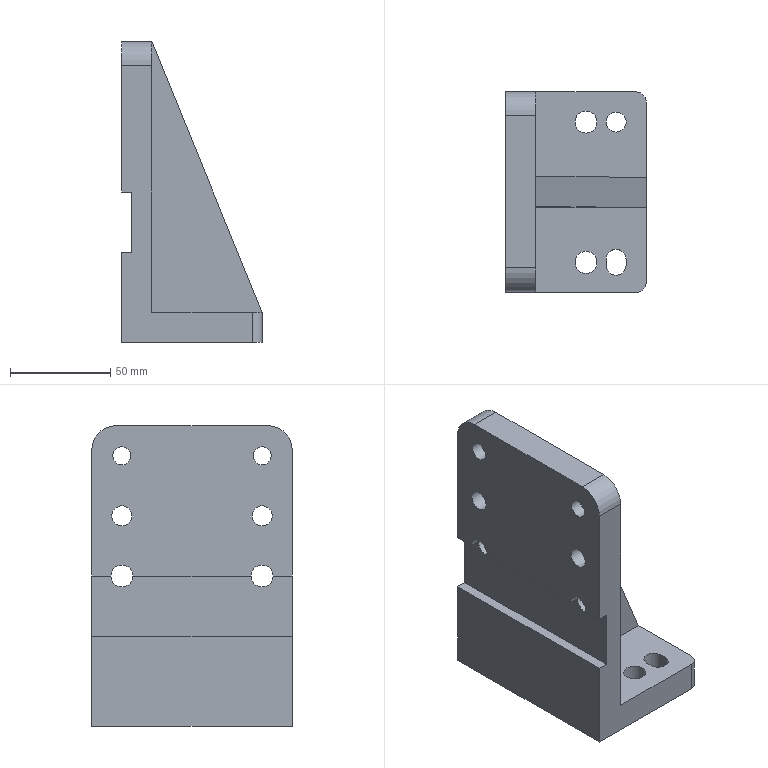Part | NX | features 5003_014_C-AIKK150-70 2 | 1 solid | 40 faces | box 70 x 100 x 150 mm | volume 332766 mm3 | plane 23 | cylinder 17 | commonest cylinder face diameters 10 x7 11 x4 9 x2 15 x2 24 x2
STEP:
#1=CARTESIAN_POINT('',(218.525,-42.5,-112.));
#2=VERTEX_POINT('',#1);
#3=CARTESIAN_POINT('',(218.525,-52.,-112.));
#4=VERTEX_POINT('',#3);
#5=CARTESIAN_POINT('',(218.525,48.,-112.));
#6=DIRECTION('',(0.,-1.,0.));
#7=VECTOR('',#6,1000.);
#8=LINE('',#5,#7);
#9=EDGE_CURVE('',#2,#4,#8,.T.);
#10=ORIENTED_EDGE('',*,*,#9,.F.);
#11=CARTESIAN_POINT('',(223.525,-42.5,-112.));
#12=VERTEX_POINT('',#11);
#13=CARTESIAN_POINT('',(233.525,-42.5,-112.));
#14=DIRECTION('',(1.,0.,0.));
#15=VECTOR('',#14,1000.);
#16=LINE('',#13,#15);
#17=EDGE_CURVE('',#2,#12,#16,.T.);
#18=ORIENTED_EDGE('',*,*,#17,.T.);
#19=CARTESIAN_POINT('',(223.525,-52.,-112.));
#20=VERTEX_POINT('',#19);
#21=CARTESIAN_POINT('',(223.525,48.,-112.));
#22=DIRECTION('',(0.,-1.,0.));
#23=VECTOR('',#22,1000.);
#24=LINE('',#21,#23);
#25=EDGE_CURVE('',#12,#20,#24,.T.);
#26=ORIENTED_EDGE('',*,*,#25,.T.);
#27=CARTESIAN_POINT('',(218.525,-52.,-112.));
#28=DIRECTION('',(-1.,0.,0.));
#29=VECTOR('',#28,1000.);
#30=LINE('',#27,#29);
#31=EDGE_CURVE('',#20,#4,#30,.T.);
#32=ORIENTED_EDGE('',*,*,#31,.T.);
#33=EDGE_LOOP('',(#10,#18,#26,#32));
#34=FACE_BOUND('',#33,.T.);
#35=CARTESIAN_POINT('',(218.525,48.,-112.));
#36=DIRECTION('',(0.,0.,1.));
#37=DIRECTION('',(0.,-1.,0.));
#38=AXIS2_PLACEMENT_3D('',#35,#36,#37);
#39=PLANE('',#38);
#40=ADVANCED_FACE('',(#34),#39,.F.);
#41=CARTESIAN_POINT('',(223.525,27.5,-112.));
#42=VERTEX_POINT('',#41);
#43=CARTESIAN_POINT('',(223.525,-31.5,-112.));
#44=VERTEX_POINT('',#43);
#45=CARTESIAN_POINT('',(223.525,48.,-112.));
#46=DIRECTION('',(0.,-1.,0.));
#47=VECTOR('',#46,1000.);
#48=LINE('',#45,#47);
#49=EDGE_CURVE('',#42,#44,#48,.T.);
#50=ORIENTED_EDGE('',*,*,#49,.T.);
#51=CARTESIAN_POINT('',(218.525,-31.5,-112.));
#52=VERTEX_POINT('',#51);
#53=CARTESIAN_POINT('',(233.525,-31.5,-112.));
#54=DIRECTION('',(1.,0.,0.));
#55=VECTOR('',#54,1000.);
#56=LINE('',#53,#55);
#57=EDGE_CURVE('',#44,#52,#56,.F.);
#58=ORIENTED_EDGE('',*,*,#57,.T.);
#59=CARTESIAN_POINT('',(218.525,27.5,-112.));
#60=VERTEX_POINT('',#59);
#61=CARTESIAN_POINT('',(218.525,48.,-112.));
#62=DIRECTION('',(0.,-1.,0.));
#63=VECTOR('',#62,1000.);
#64=LINE('',#61,#63);
#65=EDGE_CURVE('',#60,#52,#64,.T.);
#66=ORIENTED_EDGE('',*,*,#65,.F.);
#67=CARTESIAN_POINT('',(233.525,27.5,-112.));
#68=DIRECTION('',(1.,0.,0.));
#69=VECTOR('',#68,1000.);
#70=LINE('',#67,#69);
#71=EDGE_CURVE('',#60,#42,#70,.T.);
#72=ORIENTED_EDGE('',*,*,#71,.T.);
#73=EDGE_LOOP('',(#50,#58,#66,#72));
#74=FACE_BOUND('',#73,.T.);
#75=CARTESIAN_POINT('',(218.525,48.,-112.));
#76=DIRECTION('',(0.,0.,1.));
#77=DIRECTION('',(0.,-1.,0.));
#78=AXIS2_PLACEMENT_3D('',#75,#76,#77);
#79=PLANE('',#78);
#80=ADVANCED_FACE('',(#74),#79,.F.);
#81=CARTESIAN_POINT('',(218.525,-32.,-82.));
#82=VERTEX_POINT('',#81);
#83=CARTESIAN_POINT('',(218.525,-37.,-82.));
#84=DIRECTION('',(1.,0.,0.));
#85=DIRECTION('',(0.,1.,0.));
#86=AXIS2_PLACEMENT_3D('',#83,#84,#85);
#87=CIRCLE('',#86,5.);
#88=EDGE_CURVE('',#82,#82,#87,.T.);
#89=ORIENTED_EDGE('',*,*,#88,.T.);
#90=EDGE_LOOP('',(#89));
#91=FACE_BOUND('',#90,.T.);
#92=CARTESIAN_POINT('',(218.525,38.,-82.));
#93=VERTEX_POINT('',#92);
#94=CARTESIAN_POINT('',(218.525,33.,-82.));
#95=DIRECTION('',(1.,0.,0.));
#96=DIRECTION('',(0.,1.,0.));
#97=AXIS2_PLACEMENT_3D('',#94,#95,#96);
#98=CIRCLE('',#97,5.);
#99=EDGE_CURVE('',#93,#93,#98,.T.);
#100=ORIENTED_EDGE('',*,*,#99,.T.);
#101=EDGE_LOOP('',(#100));
#102=FACE_BOUND('',#101,.T.);
#103=CARTESIAN_POINT('',(218.525,-32.5,-52.));
#104=VERTEX_POINT('',#103);
#105=CARTESIAN_POINT('',(218.525,-37.,-52.));
#106=DIRECTION('',(1.,0.,0.));
#107=DIRECTION('',(0.,1.,0.));
#108=AXIS2_PLACEMENT_3D('',#105,#106,#107);
#109=CIRCLE('',#108,4.5);
#110=EDGE_CURVE('',#104,#104,#109,.T.);
#111=ORIENTED_EDGE('',*,*,#110,.T.);
#112=EDGE_LOOP('',(#111));
#113=FACE_BOUND('',#112,.T.);
#114=CARTESIAN_POINT('',(218.525,37.5,-52.));
#115=VERTEX_POINT('',#114);
#116=CARTESIAN_POINT('',(218.525,33.,-52.));
#117=DIRECTION('',(1.,0.,0.));
#118=DIRECTION('',(0.,1.,0.));
#119=AXIS2_PLACEMENT_3D('',#116,#117,#118);
#120=CIRCLE('',#119,4.5);
#121=EDGE_CURVE('',#115,#115,#120,.T.);
#122=ORIENTED_EDGE('',*,*,#121,.T.);
#123=EDGE_LOOP('',(#122));
#124=FACE_BOUND('',#123,.T.);
#125=CARTESIAN_POINT('',(218.525,-40.,-37.));
#126=VERTEX_POINT('',#125);
#127=CARTESIAN_POINT('',(218.525,36.,-37.));
#128=VERTEX_POINT('',#127);
#129=CARTESIAN_POINT('',(218.525,-52.,-37.));
#130=DIRECTION('',(0.,1.,0.));
#131=VECTOR('',#130,1000.);
#132=LINE('',#129,#131);
#133=EDGE_CURVE('',#126,#128,#132,.T.);
#134=ORIENTED_EDGE('',*,*,#133,.T.);
#135=CARTESIAN_POINT('',(218.525,48.,-49.));
#136=VERTEX_POINT('',#135);
#137=CARTESIAN_POINT('',(218.525,36.,-49.));
#138=DIRECTION('',(1.,0.,0.));
#139=DIRECTION('',(0.,0.,1.));
#140=AXIS2_PLACEMENT_3D('',#137,#138,#139);
#141=CIRCLE('',#140,12.);
#142=EDGE_CURVE('',#128,#136,#141,.F.);
#143=ORIENTED_EDGE('',*,*,#142,.T.);
#144=CARTESIAN_POINT('',(218.525,48.,-112.));
#145=VERTEX_POINT('',#144);
#146=CARTESIAN_POINT('',(218.525,48.,-37.));
#147=DIRECTION('',(0.,0.,-1.));
#148=VECTOR('',#147,1000.);
#149=LINE('',#146,#148);
#150=EDGE_CURVE('',#136,#145,#149,.T.);
#151=ORIENTED_EDGE('',*,*,#150,.T.);
#152=CARTESIAN_POINT('',(218.525,38.5,-112.));
#153=VERTEX_POINT('',#152);
#154=CARTESIAN_POINT('',(218.525,48.,-112.));
#155=DIRECTION('',(0.,-1.,0.));
#156=VECTOR('',#155,1000.);
#157=LINE('',#154,#156);
#158=EDGE_CURVE('',#145,#153,#157,.T.);
#159=ORIENTED_EDGE('',*,*,#158,.T.);
#160=CARTESIAN_POINT('',(218.525,33.,-112.));
#161=DIRECTION('',(1.,0.,0.));
#162=DIRECTION('',(0.,1.,0.));
#163=AXIS2_PLACEMENT_3D('',#160,#161,#162);
#164=CIRCLE('',#163,5.5);
#165=EDGE_CURVE('',#153,#60,#164,.T.);
#166=ORIENTED_EDGE('',*,*,#165,.T.);
#167=ORIENTED_EDGE('',*,*,#65,.T.);
#168=CARTESIAN_POINT('',(218.525,-37.,-112.));
#169=DIRECTION('',(1.,0.,0.));
#170=DIRECTION('',(0.,1.,0.));
#171=AXIS2_PLACEMENT_3D('',#168,#169,#170);
#172=CIRCLE('',#171,5.5);
#173=EDGE_CURVE('',#52,#2,#172,.T.);
#174=ORIENTED_EDGE('',*,*,#173,.T.);
#175=ORIENTED_EDGE('',*,*,#9,.T.);
#176=CARTESIAN_POINT('',(218.525,-52.,-49.));
#177=VERTEX_POINT('',#176);
#178=CARTESIAN_POINT('',(218.525,-52.,-37.));
#179=DIRECTION('',(0.,0.,-1.));
#180=VECTOR('',#179,1000.);
#181=LINE('',#178,#180);
#182=EDGE_CURVE('',#177,#4,#181,.T.);
#183=ORIENTED_EDGE('',*,*,#182,.F.);
#184=CARTESIAN_POINT('',(218.525,-40.,-49.));
#185=DIRECTION('',(1.,0.,0.));
#186=DIRECTION('',(0.,0.,1.));
#187=AXIS2_PLACEMENT_3D('',#184,#185,#186);
#188=CIRCLE('',#187,12.);
#189=EDGE_CURVE('',#177,#126,#188,.F.);
#190=ORIENTED_EDGE('',*,*,#189,.T.);
#191=EDGE_LOOP('',(#134,#143,#151,#159,#166,#167,#174,#175,#183,#190));
#192=FACE_BOUND('',#191,.T.);
#193=CARTESIAN_POINT('',(218.525,-52.,-37.));
#194=DIRECTION('',(1.,0.,0.));
#195=DIRECTION('',(0.,0.,1.));
#196=AXIS2_PLACEMENT_3D('',#193,#194,#195);
#197=PLANE('',#196);
#198=ADVANCED_FACE('',(#91,#102,#113,#124,#192),#197,.F.);
#199=CARTESIAN_POINT('',(218.525,-52.,-142.));
#200=VERTEX_POINT('',#199);
#201=CARTESIAN_POINT('',(218.525,-52.,-187.));
#202=VERTEX_POINT('',#201);
#203=CARTESIAN_POINT('',(218.525,-52.,-37.));
#204=DIRECTION('',(0.,0.,-1.));
#205=VECTOR('',#204,1000.);
#206=LINE('',#203,#205);
#207=EDGE_CURVE('',#200,#202,#206,.T.);
#208=ORIENTED_EDGE('',*,*,#207,.F.);
#209=CARTESIAN_POINT('',(218.525,48.,-142.));
#210=VERTEX_POINT('',#209);
#211=CARTESIAN_POINT('',(218.525,48.,-142.));
#212=DIRECTION('',(0.,-1.,0.));
#213=VECTOR('',#212,1000.);
#214=LINE('',#211,#213);
#215=EDGE_CURVE('',#210,#200,#214,.T.);
#216=ORIENTED_EDGE('',*,*,#215,.F.);
#217=CARTESIAN_POINT('',(218.525,48.,-187.));
#218=VERTEX_POINT('',#217);
#219=CARTESIAN_POINT('',(218.525,48.,-37.));
#220=DIRECTION('',(0.,0.,-1.));
#221=VECTOR('',#220,1000.);
#222=LINE('',#219,#221);
#223=EDGE_CURVE('',#210,#218,#222,.T.);
#224=ORIENTED_EDGE('',*,*,#223,.T.);
#225=CARTESIAN_POINT('',(218.525,-52.,-187.));
#226=DIRECTION('',(0.,1.,0.));
#227=VECTOR('',#226,1000.);
#228=LINE('',#225,#227);
#229=EDGE_CURVE('',#202,#218,#228,.T.);
#230=ORIENTED_EDGE('',*,*,#229,.F.);
#231=EDGE_LOOP('',(#208,#216,#224,#230));
#232=FACE_BOUND('',#231,.T.);
#233=CARTESIAN_POINT('',(218.525,-52.,-37.));
#234=DIRECTION('',(1.,0.,0.));
#235=DIRECTION('',(0.,0.,1.));
#236=AXIS2_PLACEMENT_3D('',#233,#234,#235);
#237=PLANE('',#236);
#238=ADVANCED_FACE('',(#232),#237,.F.);
#239=CARTESIAN_POINT('',(268.525,-38.5,-187.));
#240=VERTEX_POINT('',#239);
#241=CARTESIAN_POINT('',(268.525,-35.5,-187.));
#242=VERTEX_POINT('',#241);
#243=CARTESIAN_POINT('',(268.525,-38.5,-187.));
#244=DIRECTION('',(0.,1.,0.));
#245=VECTOR('',#244,1000.);
#246=LINE('',#243,#245);
#247=EDGE_CURVE('',#240,#242,#246,.T.);
#248=ORIENTED_EDGE('',*,*,#247,.F.);
#249=CARTESIAN_POINT('',(278.525,-38.5,-187.));
#250=VERTEX_POINT('',#249);
#251=CARTESIAN_POINT('',(273.525,-38.5,-187.));
#252=DIRECTION('',(0.,0.,1.));
#253=DIRECTION('',(0.,-1.,0.));
#254=AXIS2_PLACEMENT_3D('',#251,#252,#253);
#255=CIRCLE('',#254,5.);
#256=EDGE_CURVE('',#240,#250,#255,.T.);
#257=ORIENTED_EDGE('',*,*,#256,.T.);
#258=CARTESIAN_POINT('',(278.525,-35.5,-187.));
#259=VERTEX_POINT('',#258);
#260=CARTESIAN_POINT('',(278.525,-38.5,-187.));
#261=DIRECTION('',(0.,1.,0.));
#262=VECTOR('',#261,1000.);
#263=LINE('',#260,#262);
#264=EDGE_CURVE('',#250,#259,#263,.T.);
#265=ORIENTED_EDGE('',*,*,#264,.T.);
#266=CARTESIAN_POINT('',(273.525,-35.5,-187.));
#267=DIRECTION('',(0.,0.,1.));
#268=DIRECTION('',(0.,-1.,0.));
#269=AXIS2_PLACEMENT_3D('',#266,#267,#268);
#270=CIRCLE('',#269,5.);
#271=EDGE_CURVE('',#259,#242,#270,.T.);
#272=ORIENTED_EDGE('',*,*,#271,.T.);
#273=EDGE_LOOP('',(#248,#257,#265,#272));
#274=FACE_BOUND('',#273,.T.);
#275=CARTESIAN_POINT('',(258.525,27.5,-187.));
#276=VERTEX_POINT('',#275);
#277=CARTESIAN_POINT('',(258.525,33.,-187.));
#278=DIRECTION('',(0.,0.,1.));
#279=DIRECTION('',(0.,-1.,0.));
#280=AXIS2_PLACEMENT_3D('',#277,#278,#279);
#281=CIRCLE('',#280,5.5);
#282=EDGE_CURVE('',#276,#276,#281,.T.);
#283=ORIENTED_EDGE('',*,*,#282,.T.);
#284=EDGE_LOOP('',(#283));
#285=FACE_BOUND('',#284,.T.);
#286=CARTESIAN_POINT('',(258.525,-42.5,-187.));
#287=VERTEX_POINT('',#286);
#288=CARTESIAN_POINT('',(258.525,-37.,-187.));
#289=DIRECTION('',(0.,0.,1.));
#290=DIRECTION('',(0.,-1.,0.));
#291=AXIS2_PLACEMENT_3D('',#288,#289,#290);
#292=CIRCLE('',#291,5.5);
#293=EDGE_CURVE('',#287,#287,#292,.T.);
#294=ORIENTED_EDGE('',*,*,#293,.T.);
#295=EDGE_LOOP('',(#294));
#296=FACE_BOUND('',#295,.T.);
#297=CARTESIAN_POINT('',(273.525,28.,-187.));
#298=VERTEX_POINT('',#297);
#299=CARTESIAN_POINT('',(273.525,33.,-187.));
#300=DIRECTION('',(0.,0.,1.));
#301=DIRECTION('',(0.,-1.,0.));
#302=AXIS2_PLACEMENT_3D('',#299,#300,#301);
#303=CIRCLE('',#302,5.);
#304=EDGE_CURVE('',#298,#298,#303,.T.);
#305=ORIENTED_EDGE('',*,*,#304,.T.);
#306=EDGE_LOOP('',(#305));
#307=FACE_BOUND('',#306,.T.);
#308=CARTESIAN_POINT('',(283.525,48.,-187.));
#309=VERTEX_POINT('',#308);
#310=CARTESIAN_POINT('',(218.525,48.,-187.));
#311=DIRECTION('',(1.,0.,0.));
#312=VECTOR('',#311,1000.);
#313=LINE('',#310,#312);
#314=EDGE_CURVE('',#218,#309,#313,.T.);
#315=ORIENTED_EDGE('',*,*,#314,.T.);
#316=CARTESIAN_POINT('',(288.525,43.,-187.));
#317=VERTEX_POINT('',#316);
#318=CARTESIAN_POINT('',(283.525,43.,-187.));
#319=DIRECTION('',(0.,0.,1.));
#320=DIRECTION('',(0.,-1.,0.));
#321=AXIS2_PLACEMENT_3D('',#318,#319,#320);
#322=CIRCLE('',#321,5.);
#323=EDGE_CURVE('',#309,#317,#322,.F.);
#324=ORIENTED_EDGE('',*,*,#323,.T.);
#325=CARTESIAN_POINT('',(288.525,-47.,-187.));
#326=VERTEX_POINT('',#325);
#327=CARTESIAN_POINT('',(288.525,-52.,-187.));
#328=DIRECTION('',(0.,1.,0.));
#329=VECTOR('',#328,1000.);
#330=LINE('',#327,#329);
#331=EDGE_CURVE('',#326,#317,#330,.T.);
#332=ORIENTED_EDGE('',*,*,#331,.F.);
#333=CARTESIAN_POINT('',(283.525,-52.,-187.));
#334=VERTEX_POINT('',#333);
#335=CARTESIAN_POINT('',(283.525,-47.,-187.));
#336=DIRECTION('',(0.,0.,1.));
#337=DIRECTION('',(0.,-1.,0.));
#338=AXIS2_PLACEMENT_3D('',#335,#336,#337);
#339=CIRCLE('',#338,5.);
#340=EDGE_CURVE('',#326,#334,#339,.F.);
#341=ORIENTED_EDGE('',*,*,#340,.T.);
#342=CARTESIAN_POINT('',(218.525,-52.,-187.));
#343=DIRECTION('',(1.,0.,0.));
#344=VECTOR('',#343,1000.);
#345=LINE('',#342,#344);
#346=EDGE_CURVE('',#202,#334,#345,.T.);
#347=ORIENTED_EDGE('',*,*,#346,.F.);
#348=ORIENTED_EDGE('',*,*,#229,.T.);
#349=EDGE_LOOP('',(#315,#324,#332,#341,#347,#348));
#350=FACE_BOUND('',#349,.T.);
#351=CARTESIAN_POINT('',(218.525,-52.,-187.));
#352=DIRECTION('',(0.,0.,1.));
#353=DIRECTION('',(0.,-1.,0.));
#354=AXIS2_PLACEMENT_3D('',#351,#352,#353);
#355=PLANE('',#354);
#356=ADVANCED_FACE('',(#274,#285,#296,#307,#350),#355,.F.);
#357=ORIENTED_EDGE('',*,*,#331,.T.);
#358=CARTESIAN_POINT('',(288.525,43.,-172.));
#359=VERTEX_POINT('',#358);
#360=CARTESIAN_POINT('',(288.525,43.,-187.));
#361=DIRECTION('',(0.,0.,1.));
#362=VECTOR('',#361,1000.);
#363=LINE('',#360,#362);
#364=EDGE_CURVE('',#317,#359,#363,.T.);
#365=ORIENTED_EDGE('',*,*,#364,.T.);
#366=CARTESIAN_POINT('',(288.525,5.5,-172.));
#367=VERTEX_POINT('',#366);
#368=CARTESIAN_POINT('',(288.525,48.,-172.));
#369=DIRECTION('',(0.,1.,0.));
#370=VECTOR('',#369,1000.);
#371=LINE('',#368,#370);
#372=EDGE_CURVE('',#367,#359,#371,.T.);
#373=ORIENTED_EDGE('',*,*,#372,.F.);
#374=CARTESIAN_POINT('',(288.525,-9.5,-172.));
#375=VERTEX_POINT('',#374);
#376=CARTESIAN_POINT('',(288.525,-52.,-172.));
#377=DIRECTION('',(0.,1.,0.));
#378=VECTOR('',#377,1000.);
#379=LINE('',#376,#378);
#380=EDGE_CURVE('',#375,#367,#379,.T.);
#381=ORIENTED_EDGE('',*,*,#380,.F.);
#382=CARTESIAN_POINT('',(288.525,-47.,-172.));
#383=VERTEX_POINT('',#382);
#384=CARTESIAN_POINT('',(288.525,-52.,-172.));
#385=DIRECTION('',(0.,1.,0.));
#386=VECTOR('',#385,1000.);
#387=LINE('',#384,#386);
#388=EDGE_CURVE('',#383,#375,#387,.T.);
#389=ORIENTED_EDGE('',*,*,#388,.F.);
#390=CARTESIAN_POINT('',(288.525,-47.,-187.));
#391=DIRECTION('',(0.,0.,1.));
#392=VECTOR('',#391,1000.);
#393=LINE('',#390,#392);
#394=EDGE_CURVE('',#383,#326,#393,.F.);
#395=ORIENTED_EDGE('',*,*,#394,.T.);
#396=EDGE_LOOP('',(#357,#365,#373,#381,#389,#395));
#397=FACE_BOUND('',#396,.T.);
#398=CARTESIAN_POINT('',(288.525,-52.,-187.));
#399=DIRECTION('',(-1.,0.,0.));
#400=DIRECTION('',(0.,-1.,0.));
#401=AXIS2_PLACEMENT_3D('',#398,#399,#400);
#402=PLANE('',#401);
#403=ADVANCED_FACE('',(#397),#402,.F.);
#404=CARTESIAN_POINT('',(233.525,-9.5,-37.));
#405=VERTEX_POINT('',#404);
#406=CARTESIAN_POINT('',(233.525,5.5,-37.));
#407=VERTEX_POINT('',#406);
#408=CARTESIAN_POINT('',(233.525,-52.,-37.));
#409=DIRECTION('',(0.,1.,0.));
#410=VECTOR('',#409,1000.);
#411=LINE('',#408,#410);
#412=EDGE_CURVE('',#405,#407,#411,.T.);
#413=ORIENTED_EDGE('',*,*,#412,.F.);
#414=CARTESIAN_POINT('',(233.525,-9.5,-37.));
#415=DIRECTION('',(0.3773,0.,-0.9261));
#416=VECTOR('',#415,1000.);
#417=LINE('',#414,#416);
#418=EDGE_CURVE('',#405,#375,#417,.T.);
#419=ORIENTED_EDGE('',*,*,#418,.T.);
#420=ORIENTED_EDGE('',*,*,#380,.T.);
#421=CARTESIAN_POINT('',(233.525,5.5,-37.));
#422=DIRECTION('',(-0.3773,0.,0.9261));
#423=VECTOR('',#422,1000.);
#424=LINE('',#421,#423);
#425=EDGE_CURVE('',#367,#407,#424,.T.);
#426=ORIENTED_EDGE('',*,*,#425,.T.);
#427=EDGE_LOOP('',(#413,#419,#420,#426));
#428=FACE_BOUND('',#427,.T.);
#429=CARTESIAN_POINT('',(233.525,-52.,-37.));
#430=DIRECTION('',(-0.9261,0.,-0.3773));
#431=DIRECTION('',(0.3773,0.,-0.9261));
#432=AXIS2_PLACEMENT_3D('',#429,#430,#431);
#433=PLANE('',#432);
#434=ADVANCED_FACE('',(#428),#433,.F.);
#435=CARTESIAN_POINT('',(233.525,36.,-37.));
#436=VERTEX_POINT('',#435);
#437=CARTESIAN_POINT('',(233.525,48.,-37.));
#438=DIRECTION('',(0.,-1.,0.));
#439=VECTOR('',#438,1000.);
#440=LINE('',#437,#439);
#441=EDGE_CURVE('',#436,#407,#440,.T.);
#442=ORIENTED_EDGE('',*,*,#441,.F.);
#443=CARTESIAN_POINT('',(233.525,36.,-37.));
#444=DIRECTION('',(-1.,0.,0.));
#445=VECTOR('',#444,1000.);
#446=LINE('',#443,#445);
#447=EDGE_CURVE('',#436,#128,#446,.T.);
#448=ORIENTED_EDGE('',*,*,#447,.T.);
#449=ORIENTED_EDGE('',*,*,#133,.F.);
#450=CARTESIAN_POINT('',(233.525,-40.,-37.));
#451=VERTEX_POINT('',#450);
#452=CARTESIAN_POINT('',(233.525,-40.,-37.));
#453=DIRECTION('',(-1.,0.,0.));
#454=VECTOR('',#453,1000.);
#455=LINE('',#452,#454);
#456=EDGE_CURVE('',#126,#451,#455,.F.);
#457=ORIENTED_EDGE('',*,*,#456,.T.);
#458=CARTESIAN_POINT('',(233.525,-52.,-37.));
#459=DIRECTION('',(0.,1.,0.));
#460=VECTOR('',#459,1000.);
#461=LINE('',#458,#460);
#462=EDGE_CURVE('',#451,#405,#461,.T.);
#463=ORIENTED_EDGE('',*,*,#462,.T.);
#464=ORIENTED_EDGE('',*,*,#412,.T.);
#465=EDGE_LOOP('',(#442,#448,#449,#457,#463,#464));
#466=FACE_BOUND('',#465,.T.);
#467=CARTESIAN_POINT('',(233.525,-52.,-37.));
#468=DIRECTION('',(0.,0.,-1.));
#469=DIRECTION('',(0.,1.,0.));
#470=AXIS2_PLACEMENT_3D('',#467,#468,#469);
#471=PLANE('',#470);
#472=ADVANCED_FACE('',(#466),#471,.F.);
#473=ORIENTED_EDGE('',*,*,#346,.T.);
#474=CARTESIAN_POINT('',(283.525,-52.,-172.));
#475=VERTEX_POINT('',#474);
#476=CARTESIAN_POINT('',(283.525,-52.,-172.));
#477=DIRECTION('',(0.,0.,1.));
#478=VECTOR('',#477,1000.);
#479=LINE('',#476,#478);
#480=EDGE_CURVE('',#334,#475,#479,.T.);
#481=ORIENTED_EDGE('',*,*,#480,.T.);
#482=CARTESIAN_POINT('',(233.525,-52.,-172.));
#483=VERTEX_POINT('',#482);
#484=CARTESIAN_POINT('',(233.525,-52.,-172.));
#485=DIRECTION('',(1.,0.,0.));
#486=VECTOR('',#485,1000.);
#487=LINE('',#484,#486);
#488=EDGE_CURVE('',#483,#475,#487,.T.);
#489=ORIENTED_EDGE('',*,*,#488,.F.);
#490=CARTESIAN_POINT('',(233.525,-52.,-49.));
#491=VERTEX_POINT('',#490);
#492=CARTESIAN_POINT('',(233.525,-52.,-172.));
#493=DIRECTION('',(0.,0.,1.));
#494=VECTOR('',#493,1000.);
#495=LINE('',#492,#494);
#496=EDGE_CURVE('',#483,#491,#495,.T.);
#497=ORIENTED_EDGE('',*,*,#496,.T.);
#498=CARTESIAN_POINT('',(218.525,-52.,-49.));
#499=DIRECTION('',(-1.,0.,0.));
#500=VECTOR('',#499,1000.);
#501=LINE('',#498,#500);
#502=EDGE_CURVE('',#491,#177,#501,.T.);
#503=ORIENTED_EDGE('',*,*,#502,.T.);
#504=ORIENTED_EDGE('',*,*,#182,.T.);
#505=ORIENTED_EDGE('',*,*,#31,.F.);
#506=CARTESIAN_POINT('',(223.525,-52.,-142.));
#507=VERTEX_POINT('',#506);
#508=CARTESIAN_POINT('',(223.525,-52.,-112.));
#509=DIRECTION('',(0.,0.,1.));
#510=VECTOR('',#509,1000.);
#511=LINE('',#508,#510);
#512=EDGE_CURVE('',#507,#20,#511,.T.);
#513=ORIENTED_EDGE('',*,*,#512,.F.);
#514=CARTESIAN_POINT('',(223.525,-52.,-142.));
#515=DIRECTION('',(1.,0.,0.));
#516=VECTOR('',#515,1000.);
#517=LINE('',#514,#516);
#518=EDGE_CURVE('',#200,#507,#517,.T.);
#519=ORIENTED_EDGE('',*,*,#518,.F.);
#520=ORIENTED_EDGE('',*,*,#207,.T.);
#521=EDGE_LOOP('',(#473,#481,#489,#497,#503,#504,#505,#513,#519,#520));
#522=FACE_BOUND('',#521,.T.);
#523=CARTESIAN_POINT('',(218.525,-52.,-187.));
#524=DIRECTION('',(0.,-1.,0.));
#525=DIRECTION('',(1.,0.,0.));
#526=AXIS2_PLACEMENT_3D('',#523,#524,#525);
#527=PLANE('',#526);
#528=ADVANCED_FACE('',(#522),#527,.T.);
#529=CARTESIAN_POINT('',(283.525,48.,-172.));
#530=VERTEX_POINT('',#529);
#531=CARTESIAN_POINT('',(233.525,48.,-172.));
#532=VERTEX_POINT('',#531);
#533=CARTESIAN_POINT('',(288.525,48.,-172.));
#534=DIRECTION('',(-1.,0.,0.));
#535=VECTOR('',#534,1000.);
#536=LINE('',#533,#535);
#537=EDGE_CURVE('',#530,#532,#536,.T.);
#538=ORIENTED_EDGE('',*,*,#537,.F.);
#539=CARTESIAN_POINT('',(283.525,48.,-187.));
#540=DIRECTION('',(0.,0.,1.));
#541=VECTOR('',#540,1000.);
#542=LINE('',#539,#541);
#543=EDGE_CURVE('',#530,#309,#542,.F.);
#544=ORIENTED_EDGE('',*,*,#543,.T.);
#545=ORIENTED_EDGE('',*,*,#314,.F.);
#546=ORIENTED_EDGE('',*,*,#223,.F.);
#547=CARTESIAN_POINT('',(223.525,48.,-142.));
#548=VERTEX_POINT('',#547);
#549=CARTESIAN_POINT('',(223.525,48.,-142.));
#550=DIRECTION('',(1.,0.,0.));
#551=VECTOR('',#550,1000.);
#552=LINE('',#549,#551);
#553=EDGE_CURVE('',#210,#548,#552,.T.);
#554=ORIENTED_EDGE('',*,*,#553,.T.);
#555=CARTESIAN_POINT('',(223.525,48.,-112.));
#556=VERTEX_POINT('',#555);
#557=CARTESIAN_POINT('',(223.525,48.,-112.));
#558=DIRECTION('',(0.,0.,1.));
#559=VECTOR('',#558,1000.);
#560=LINE('',#557,#559);
#561=EDGE_CURVE('',#548,#556,#560,.T.);
#562=ORIENTED_EDGE('',*,*,#561,.T.);
#563=CARTESIAN_POINT('',(218.525,48.,-112.));
#564=DIRECTION('',(-1.,0.,0.));
#565=VECTOR('',#564,1000.);
#566=LINE('',#563,#565);
#567=EDGE_CURVE('',#556,#145,#566,.T.);
#568=ORIENTED_EDGE('',*,*,#567,.T.);
#569=ORIENTED_EDGE('',*,*,#150,.F.);
#570=CARTESIAN_POINT('',(233.525,48.,-49.));
#571=VERTEX_POINT('',#570);
#572=CARTESIAN_POINT('',(218.525,48.,-49.));
#573=DIRECTION('',(-1.,0.,0.));
#574=VECTOR('',#573,1000.);
#575=LINE('',#572,#574);
#576=EDGE_CURVE('',#136,#571,#575,.F.);
#577=ORIENTED_EDGE('',*,*,#576,.T.);
#578=CARTESIAN_POINT('',(233.525,48.,-172.));
#579=DIRECTION('',(0.,0.,1.));
#580=VECTOR('',#579,1000.);
#581=LINE('',#578,#580);
#582=EDGE_CURVE('',#532,#571,#581,.T.);
#583=ORIENTED_EDGE('',*,*,#582,.F.);
#584=EDGE_LOOP('',(#538,#544,#545,#546,#554,#562,#568,#569,#577,#583));
#585=FACE_BOUND('',#584,.T.);
#586=CARTESIAN_POINT('',(218.525,48.,-187.));
#587=DIRECTION('',(0.,-1.,0.));
#588=DIRECTION('',(1.,0.,0.));
#589=AXIS2_PLACEMENT_3D('',#586,#587,#588);
#590=PLANE('',#589);
#591=ADVANCED_FACE('',(#585),#590,.F.);
#592=CARTESIAN_POINT('',(223.525,38.5,-112.));
#593=VERTEX_POINT('',#592);
#594=CARTESIAN_POINT('',(223.525,48.,-112.));
#595=DIRECTION('',(0.,-1.,0.));
#596=VECTOR('',#595,1000.);
#597=LINE('',#594,#596);
#598=EDGE_CURVE('',#556,#593,#597,.T.);
#599=ORIENTED_EDGE('',*,*,#598,.T.);
#600=CARTESIAN_POINT('',(233.525,38.5,-112.));
#601=DIRECTION('',(1.,0.,0.));
#602=VECTOR('',#601,1000.);
#603=LINE('',#600,#602);
#604=EDGE_CURVE('',#593,#153,#603,.F.);
#605=ORIENTED_EDGE('',*,*,#604,.T.);
#606=ORIENTED_EDGE('',*,*,#158,.F.);
#607=ORIENTED_EDGE('',*,*,#567,.F.);
#608=EDGE_LOOP('',(#599,#605,#606,#607));
#609=FACE_BOUND('',#608,.T.);
#610=CARTESIAN_POINT('',(218.525,48.,-112.));
#611=DIRECTION('',(0.,0.,1.));
#612=DIRECTION('',(0.,-1.,0.));
#613=AXIS2_PLACEMENT_3D('',#610,#611,#612);
#614=PLANE('',#613);
#615=ADVANCED_FACE('',(#609),#614,.F.);
#616=ORIENTED_EDGE('',*,*,#25,.F.);
#617=CARTESIAN_POINT('',(223.525,-37.,-112.));
#618=DIRECTION('',(1.,0.,0.));
#619=DIRECTION('',(0.,0.,1.));
#620=AXIS2_PLACEMENT_3D('',#617,#618,#619);
#621=CIRCLE('',#620,5.5);
#622=EDGE_CURVE('',#12,#44,#621,.T.);
#623=ORIENTED_EDGE('',*,*,#622,.T.);
#624=ORIENTED_EDGE('',*,*,#49,.F.);
#625=CARTESIAN_POINT('',(223.525,33.,-112.));
#626=DIRECTION('',(1.,0.,0.));
#627=DIRECTION('',(0.,0.,1.));
#628=AXIS2_PLACEMENT_3D('',#625,#626,#627);
#629=CIRCLE('',#628,5.5);
#630=EDGE_CURVE('',#42,#593,#629,.T.);
#631=ORIENTED_EDGE('',*,*,#630,.T.);
#632=ORIENTED_EDGE('',*,*,#598,.F.);
#633=ORIENTED_EDGE('',*,*,#561,.F.);
#634=CARTESIAN_POINT('',(223.525,48.,-142.));
#635=DIRECTION('',(0.,-1.,0.));
#636=VECTOR('',#635,1000.);
#637=LINE('',#634,#636);
#638=EDGE_CURVE('',#548,#507,#637,.T.);
#639=ORIENTED_EDGE('',*,*,#638,.T.);
#640=ORIENTED_EDGE('',*,*,#512,.T.);
#641=EDGE_LOOP('',(#616,#623,#624,#631,#632,#633,#639,#640));
#642=FACE_BOUND('',#641,.T.);
#643=CARTESIAN_POINT('',(223.525,48.,-112.));
#644=DIRECTION('',(1.,0.,0.));
#645=DIRECTION('',(0.,0.,1.));
#646=AXIS2_PLACEMENT_3D('',#643,#644,#645);
#647=PLANE('',#646);
#648=ADVANCED_FACE('',(#642),#647,.F.);
#649=ORIENTED_EDGE('',*,*,#518,.T.);
#650=ORIENTED_EDGE('',*,*,#638,.F.);
#651=ORIENTED_EDGE('',*,*,#553,.F.);
#652=ORIENTED_EDGE('',*,*,#215,.T.);
#653=EDGE_LOOP('',(#649,#650,#651,#652));
#654=FACE_BOUND('',#653,.T.);
#655=CARTESIAN_POINT('',(223.525,48.,-142.));
#656=DIRECTION('',(0.,0.,-1.));
#657=DIRECTION('',(0.,1.,0.));
#658=AXIS2_PLACEMENT_3D('',#655,#656,#657);
#659=PLANE('',#658);
#660=ADVANCED_FACE('',(#654),#659,.F.);
#661=CARTESIAN_POINT('',(233.525,5.5,-172.));
#662=VERTEX_POINT('',#661);
#663=CARTESIAN_POINT('',(288.525,5.5,-172.));
#664=DIRECTION('',(1.,0.,0.));
#665=VECTOR('',#664,1000.);
#666=LINE('',#663,#665);
#667=EDGE_CURVE('',#662,#367,#666,.T.);
#668=ORIENTED_EDGE('',*,*,#667,.F.);
#669=CARTESIAN_POINT('',(233.525,5.5,-172.));
#670=DIRECTION('',(0.,0.,1.));
#671=VECTOR('',#670,1000.);
#672=LINE('',#669,#671);
#673=EDGE_CURVE('',#662,#407,#672,.T.);
#674=ORIENTED_EDGE('',*,*,#673,.T.);
#675=ORIENTED_EDGE('',*,*,#425,.F.);
#676=EDGE_LOOP('',(#668,#674,#675));
#677=FACE_BOUND('',#676,.T.);
#678=CARTESIAN_POINT('',(288.525,5.5,-172.));
#679=DIRECTION('',(0.,-1.,0.));
#680=DIRECTION('',(1.,0.,0.));
#681=AXIS2_PLACEMENT_3D('',#678,#679,#680);
#682=PLANE('',#681);
#683=ADVANCED_FACE('',(#677),#682,.F.);
#684=CARTESIAN_POINT('',(233.525,38.,-82.));
#685=VERTEX_POINT('',#684);
#686=CARTESIAN_POINT('',(233.525,33.,-82.));
#687=DIRECTION('',(1.,0.,0.));
#688=DIRECTION('',(0.,1.,0.));
#689=AXIS2_PLACEMENT_3D('',#686,#687,#688);
#690=CIRCLE('',#689,5.);
#691=EDGE_CURVE('',#685,#685,#690,.T.);
#692=ORIENTED_EDGE('',*,*,#691,.F.);
#693=EDGE_LOOP('',(#692));
#694=FACE_BOUND('',#693,.T.);
#695=CARTESIAN_POINT('',(233.525,38.5,-112.));
#696=VERTEX_POINT('',#695);
#697=CARTESIAN_POINT('',(233.525,33.,-112.));
#698=DIRECTION('',(1.,0.,0.));
#699=DIRECTION('',(0.,1.,0.));
#700=AXIS2_PLACEMENT_3D('',#697,#698,#699);
#701=CIRCLE('',#700,5.5);
#702=EDGE_CURVE('',#696,#696,#701,.T.);
#703=ORIENTED_EDGE('',*,*,#702,.F.);
#704=EDGE_LOOP('',(#703));
#705=FACE_BOUND('',#704,.T.);
#706=CARTESIAN_POINT('',(233.525,40.5,-52.));
#707=VERTEX_POINT('',#706);
#708=CARTESIAN_POINT('',(233.525,33.,-52.));
#709=DIRECTION('',(1.,0.,0.));
#710=DIRECTION('',(0.,1.,0.));
#711=AXIS2_PLACEMENT_3D('',#708,#709,#710);
#712=CIRCLE('',#711,7.5);
#713=EDGE_CURVE('',#707,#707,#712,.T.);
#714=ORIENTED_EDGE('',*,*,#713,.F.);
#715=EDGE_LOOP('',(#714));
#716=FACE_BOUND('',#715,.T.);
#717=ORIENTED_EDGE('',*,*,#582,.T.);
#718=CARTESIAN_POINT('',(233.525,36.,-49.));
#719=DIRECTION('',(-1.,0.,0.));
#720=DIRECTION('',(0.,-1.,0.));
#721=AXIS2_PLACEMENT_3D('',#718,#719,#720);
#722=CIRCLE('',#721,12.);
#723=EDGE_CURVE('',#571,#436,#722,.F.);
#724=ORIENTED_EDGE('',*,*,#723,.T.);
#725=ORIENTED_EDGE('',*,*,#441,.T.);
#726=ORIENTED_EDGE('',*,*,#673,.F.);
#727=CARTESIAN_POINT('',(233.525,48.,-172.));
#728=DIRECTION('',(0.,-1.,0.));
#729=VECTOR('',#728,1000.);
#730=LINE('',#727,#729);
#731=EDGE_CURVE('',#532,#662,#730,.T.);
#732=ORIENTED_EDGE('',*,*,#731,.F.);
#733=EDGE_LOOP('',(#717,#724,#725,#726,#732));
#734=FACE_BOUND('',#733,.T.);
#735=CARTESIAN_POINT('',(233.525,48.,-172.));
#736=DIRECTION('',(-1.,0.,0.));
#737=DIRECTION('',(0.,-1.,0.));
#738=AXIS2_PLACEMENT_3D('',#735,#736,#737);
#739=PLANE('',#738);
#740=ADVANCED_FACE('',(#694,#705,#716,#734),#739,.F.);
#741=CARTESIAN_POINT('',(258.525,27.5,-172.));
#742=VERTEX_POINT('',#741);
#743=CARTESIAN_POINT('',(258.525,33.,-172.));
#744=DIRECTION('',(0.,0.,1.));
#745=DIRECTION('',(0.,-1.,0.));
#746=AXIS2_PLACEMENT_3D('',#743,#744,#745);
#747=CIRCLE('',#746,5.5);
#748=EDGE_CURVE('',#742,#742,#747,.T.);
#749=ORIENTED_EDGE('',*,*,#748,.F.);
#750=EDGE_LOOP('',(#749));
#751=FACE_BOUND('',#750,.T.);
#752=CARTESIAN_POINT('',(273.525,28.,-172.));
#753=VERTEX_POINT('',#752);
#754=CARTESIAN_POINT('',(273.525,33.,-172.));
#755=DIRECTION('',(0.,0.,1.));
#756=DIRECTION('',(0.,-1.,0.));
#757=AXIS2_PLACEMENT_3D('',#754,#755,#756);
#758=CIRCLE('',#757,5.);
#759=EDGE_CURVE('',#753,#753,#758,.T.);
#760=ORIENTED_EDGE('',*,*,#759,.F.);
#761=EDGE_LOOP('',(#760));
#762=FACE_BOUND('',#761,.T.);
#763=ORIENTED_EDGE('',*,*,#372,.T.);
#764=CARTESIAN_POINT('',(283.525,43.,-172.));
#765=DIRECTION('',(0.,0.,-1.));
#766=DIRECTION('',(0.,1.,0.));
#767=AXIS2_PLACEMENT_3D('',#764,#765,#766);
#768=CIRCLE('',#767,5.);
#769=EDGE_CURVE('',#359,#530,#768,.F.);
#770=ORIENTED_EDGE('',*,*,#769,.T.);
#771=ORIENTED_EDGE('',*,*,#537,.T.);
#772=ORIENTED_EDGE('',*,*,#731,.T.);
#773=ORIENTED_EDGE('',*,*,#667,.T.);
#774=EDGE_LOOP('',(#763,#770,#771,#772,#773));
#775=FACE_BOUND('',#774,.T.);
#776=CARTESIAN_POINT('',(218.525,-2.,-172.));
#777=DIRECTION('',(0.,0.,-1.));
#778=DIRECTION('',(0.,1.,0.));
#779=AXIS2_PLACEMENT_3D('',#776,#777,#778);
#780=PLANE('',#779);
#781=ADVANCED_FACE('',(#751,#762,#775),#780,.F.);
#782=CARTESIAN_POINT('',(233.525,-9.5,-172.));
#783=VERTEX_POINT('',#782);
#784=CARTESIAN_POINT('',(233.525,-9.5,-172.));
#785=DIRECTION('',(0.,0.,1.));
#786=VECTOR('',#785,1000.);
#787=LINE('',#784,#786);
#788=EDGE_CURVE('',#783,#405,#787,.T.);
#789=ORIENTED_EDGE('',*,*,#788,.F.);
#790=CARTESIAN_POINT('',(233.525,-9.5,-172.));
#791=DIRECTION('',(-1.,0.,0.));
#792=VECTOR('',#791,1000.);
#793=LINE('',#790,#792);
#794=EDGE_CURVE('',#375,#783,#793,.T.);
#795=ORIENTED_EDGE('',*,*,#794,.F.);
#796=ORIENTED_EDGE('',*,*,#418,.F.);
#797=EDGE_LOOP('',(#789,#795,#796));
#798=FACE_BOUND('',#797,.T.);
#799=CARTESIAN_POINT('',(233.525,-9.5,-172.));
#800=DIRECTION('',(0.,1.,0.));
#801=DIRECTION('',(-1.,0.,0.));
#802=AXIS2_PLACEMENT_3D('',#799,#800,#801);
#803=PLANE('',#802);
#804=ADVANCED_FACE('',(#798),#803,.F.);
#805=CARTESIAN_POINT('',(233.525,-32.,-82.));
#806=VERTEX_POINT('',#805);
#807=CARTESIAN_POINT('',(233.525,-37.,-82.));
#808=DIRECTION('',(1.,0.,0.));
#809=DIRECTION('',(0.,1.,0.));
#810=AXIS2_PLACEMENT_3D('',#807,#808,#809);
#811=CIRCLE('',#810,5.);
#812=EDGE_CURVE('',#806,#806,#811,.T.);
#813=ORIENTED_EDGE('',*,*,#812,.F.);
#814=EDGE_LOOP('',(#813));
#815=FACE_BOUND('',#814,.T.);
#816=CARTESIAN_POINT('',(233.525,-31.5,-112.));
#817=VERTEX_POINT('',#816);
#818=CARTESIAN_POINT('',(233.525,-37.,-112.));
#819=DIRECTION('',(1.,0.,0.));
#820=DIRECTION('',(0.,1.,0.));
#821=AXIS2_PLACEMENT_3D('',#818,#819,#820);
#822=CIRCLE('',#821,5.5);
#823=EDGE_CURVE('',#817,#817,#822,.T.);
#824=ORIENTED_EDGE('',*,*,#823,.F.);
#825=EDGE_LOOP('',(#824));
#826=FACE_BOUND('',#825,.T.);
#827=CARTESIAN_POINT('',(233.525,-29.5,-52.));
#828=VERTEX_POINT('',#827);
#829=CARTESIAN_POINT('',(233.525,-37.,-52.));
#830=DIRECTION('',(1.,0.,0.));
#831=DIRECTION('',(0.,1.,0.));
#832=AXIS2_PLACEMENT_3D('',#829,#830,#831);
#833=CIRCLE('',#832,7.5);
#834=EDGE_CURVE('',#828,#828,#833,.T.);
#835=ORIENTED_EDGE('',*,*,#834,.F.);
#836=EDGE_LOOP('',(#835));
#837=FACE_BOUND('',#836,.T.);
#838=ORIENTED_EDGE('',*,*,#462,.F.);
#839=CARTESIAN_POINT('',(233.525,-40.,-49.));
#840=DIRECTION('',(-1.,0.,0.));
#841=DIRECTION('',(0.,-1.,0.));
#842=AXIS2_PLACEMENT_3D('',#839,#840,#841);
#843=CIRCLE('',#842,12.);
#844=EDGE_CURVE('',#451,#491,#843,.F.);
#845=ORIENTED_EDGE('',*,*,#844,.T.);
#846=ORIENTED_EDGE('',*,*,#496,.F.);
#847=CARTESIAN_POINT('',(233.525,-52.,-172.));
#848=DIRECTION('',(0.,-1.,0.));
#849=VECTOR('',#848,1000.);
#850=LINE('',#847,#849);
#851=EDGE_CURVE('',#783,#483,#850,.T.);
#852=ORIENTED_EDGE('',*,*,#851,.F.);
#853=ORIENTED_EDGE('',*,*,#788,.T.);
#854=EDGE_LOOP('',(#838,#845,#846,#852,#853));
#855=FACE_BOUND('',#854,.T.);
#856=CARTESIAN_POINT('',(233.525,-52.,-172.));
#857=DIRECTION('',(-1.,0.,0.));
#858=DIRECTION('',(0.,-1.,0.));
#859=AXIS2_PLACEMENT_3D('',#856,#857,#858);
#860=PLANE('',#859);
#861=ADVANCED_FACE('',(#815,#826,#837,#855),#860,.F.);
#862=CARTESIAN_POINT('',(268.525,-38.5,-172.));
#863=VERTEX_POINT('',#862);
#864=CARTESIAN_POINT('',(278.525,-38.5,-172.));
#865=VERTEX_POINT('',#864);
#866=CARTESIAN_POINT('',(273.525,-38.5,-172.));
#867=DIRECTION('',(0.,0.,1.));
#868=DIRECTION('',(0.,-1.,0.));
#869=AXIS2_PLACEMENT_3D('',#866,#867,#868);
#870=CIRCLE('',#869,5.);
#871=EDGE_CURVE('',#863,#865,#870,.T.);
#872=ORIENTED_EDGE('',*,*,#871,.F.);
#873=CARTESIAN_POINT('',(268.525,-35.5,-172.));
#874=VERTEX_POINT('',#873);
#875=CARTESIAN_POINT('',(268.525,-38.5,-172.));
#876=DIRECTION('',(0.,1.,0.));
#877=VECTOR('',#876,1000.);
#878=LINE('',#875,#877);
#879=EDGE_CURVE('',#863,#874,#878,.T.);
#880=ORIENTED_EDGE('',*,*,#879,.T.);
#881=CARTESIAN_POINT('',(278.525,-35.5,-172.));
#882=VERTEX_POINT('',#881);
#883=CARTESIAN_POINT('',(273.525,-35.5,-172.));
#884=DIRECTION('',(0.,0.,1.));
#885=DIRECTION('',(0.,-1.,0.));
#886=AXIS2_PLACEMENT_3D('',#883,#884,#885);
#887=CIRCLE('',#886,5.);
#888=EDGE_CURVE('',#882,#874,#887,.T.);
#889=ORIENTED_EDGE('',*,*,#888,.F.);
#890=CARTESIAN_POINT('',(278.525,-38.5,-172.));
#891=DIRECTION('',(0.,1.,0.));
#892=VECTOR('',#891,1000.);
#893=LINE('',#890,#892);
#894=EDGE_CURVE('',#865,#882,#893,.T.);
#895=ORIENTED_EDGE('',*,*,#894,.F.);
#896=EDGE_LOOP('',(#872,#880,#889,#895));
#897=FACE_BOUND('',#896,.T.);
#898=CARTESIAN_POINT('',(258.525,-42.5,-172.));
#899=VERTEX_POINT('',#898);
#900=CARTESIAN_POINT('',(258.525,-37.,-172.));
#901=DIRECTION('',(0.,0.,1.));
#902=DIRECTION('',(0.,-1.,0.));
#903=AXIS2_PLACEMENT_3D('',#900,#901,#902);
#904=CIRCLE('',#903,5.5);
#905=EDGE_CURVE('',#899,#899,#904,.T.);
#906=ORIENTED_EDGE('',*,*,#905,.F.);
#907=EDGE_LOOP('',(#906));
#908=FACE_BOUND('',#907,.T.);
#909=ORIENTED_EDGE('',*,*,#488,.T.);
#910=CARTESIAN_POINT('',(283.525,-47.,-172.));
#911=DIRECTION('',(0.,0.,-1.));
#912=DIRECTION('',(0.,1.,0.));
#913=AXIS2_PLACEMENT_3D('',#910,#911,#912);
#914=CIRCLE('',#913,5.);
#915=EDGE_CURVE('',#475,#383,#914,.F.);
#916=ORIENTED_EDGE('',*,*,#915,.T.);
#917=ORIENTED_EDGE('',*,*,#388,.T.);
#918=ORIENTED_EDGE('',*,*,#794,.T.);
#919=ORIENTED_EDGE('',*,*,#851,.T.);
#920=EDGE_LOOP('',(#909,#916,#917,#918,#919));
#921=FACE_BOUND('',#920,.T.);
#922=CARTESIAN_POINT('',(218.525,-2.,-172.));
#923=DIRECTION('',(0.,0.,-1.));
#924=DIRECTION('',(0.,1.,0.));
#925=AXIS2_PLACEMENT_3D('',#922,#923,#924);
#926=PLANE('',#925);
#927=ADVANCED_FACE('',(#897,#908,#921),#926,.F.);
#928=ORIENTED_EDGE('',*,*,#121,.F.);
#929=EDGE_LOOP('',(#928));
#930=FACE_BOUND('',#929,.T.);
#931=CARTESIAN_POINT('',(224.525,37.5,-52.));
#932=VERTEX_POINT('',#931);
#933=CARTESIAN_POINT('',(224.525,33.,-52.));
#934=DIRECTION('',(1.,0.,0.));
#935=DIRECTION('',(0.,1.,0.));
#936=AXIS2_PLACEMENT_3D('',#933,#934,#935);
#937=CIRCLE('',#936,4.5);
#938=EDGE_CURVE('',#932,#932,#937,.T.);
#939=ORIENTED_EDGE('',*,*,#938,.T.);
#940=EDGE_LOOP('',(#939));
#941=FACE_BOUND('',#940,.T.);
#942=CARTESIAN_POINT('',(233.525,33.,-52.));
#943=DIRECTION('',(1.,0.,0.));
#944=DIRECTION('',(0.,1.,0.));
#945=AXIS2_PLACEMENT_3D('',#942,#943,#944);
#946=CYLINDRICAL_SURFACE('',#945,4.5);
#947=ADVANCED_FACE('',(#930,#941),#946,.F.);
#948=ORIENTED_EDGE('',*,*,#938,.F.);
#949=EDGE_LOOP('',(#948));
#950=FACE_BOUND('',#949,.T.);
#951=CARTESIAN_POINT('',(224.525,40.5,-52.));
#952=VERTEX_POINT('',#951);
#953=CARTESIAN_POINT('',(224.525,33.,-52.));
#954=DIRECTION('',(1.,0.,0.));
#955=DIRECTION('',(0.,1.,0.));
#956=AXIS2_PLACEMENT_3D('',#953,#954,#955);
#957=CIRCLE('',#956,7.5);
#958=EDGE_CURVE('',#952,#952,#957,.T.);
#959=ORIENTED_EDGE('',*,*,#958,.T.);
#960=EDGE_LOOP('',(#959));
#961=FACE_BOUND('',#960,.T.);
#962=CARTESIAN_POINT('',(224.525,33.,-47.5));
#963=DIRECTION('',(-1.,0.,0.));
#964=DIRECTION('',(0.,-1.,0.));
#965=AXIS2_PLACEMENT_3D('',#962,#963,#964);
#966=PLANE('',#965);
#967=ADVANCED_FACE('',(#950,#961),#966,.F.);
#968=ORIENTED_EDGE('',*,*,#958,.F.);
#969=EDGE_LOOP('',(#968));
#970=FACE_BOUND('',#969,.T.);
#971=ORIENTED_EDGE('',*,*,#713,.T.);
#972=EDGE_LOOP('',(#971));
#973=FACE_BOUND('',#972,.T.);
#974=CARTESIAN_POINT('',(233.525,33.,-52.));
#975=DIRECTION('',(1.,0.,0.));
#976=DIRECTION('',(0.,1.,0.));
#977=AXIS2_PLACEMENT_3D('',#974,#975,#976);
#978=CYLINDRICAL_SURFACE('',#977,7.5);
#979=ADVANCED_FACE('',(#970,#973),#978,.F.);
#980=ORIENTED_EDGE('',*,*,#110,.F.);
#981=EDGE_LOOP('',(#980));
#982=FACE_BOUND('',#981,.T.);
#983=CARTESIAN_POINT('',(224.525,-32.5,-52.));
#984=VERTEX_POINT('',#983);
#985=CARTESIAN_POINT('',(224.525,-37.,-52.));
#986=DIRECTION('',(1.,0.,0.));
#987=DIRECTION('',(0.,1.,0.));
#988=AXIS2_PLACEMENT_3D('',#985,#986,#987);
#989=CIRCLE('',#988,4.5);
#990=EDGE_CURVE('',#984,#984,#989,.T.);
#991=ORIENTED_EDGE('',*,*,#990,.T.);
#992=EDGE_LOOP('',(#991));
#993=FACE_BOUND('',#992,.T.);
#994=CARTESIAN_POINT('',(233.525,-37.,-52.));
#995=DIRECTION('',(1.,0.,0.));
#996=DIRECTION('',(0.,1.,0.));
#997=AXIS2_PLACEMENT_3D('',#994,#995,#996);
#998=CYLINDRICAL_SURFACE('',#997,4.5);
#999=ADVANCED_FACE('',(#982,#993),#998,.F.);
#1000=ORIENTED_EDGE('',*,*,#990,.F.);
#1001=EDGE_LOOP('',(#1000));
#1002=FACE_BOUND('',#1001,.T.);
#1003=CARTESIAN_POINT('',(224.525,-29.5,-52.));
#1004=VERTEX_POINT('',#1003);
#1005=CARTESIAN_POINT('',(224.525,-37.,-52.));
#1006=DIRECTION('',(1.,0.,0.));
#1007=DIRECTION('',(0.,1.,0.));
#1008=AXIS2_PLACEMENT_3D('',#1005,#1006,#1007);
#1009=CIRCLE('',#1008,7.5);
#1010=EDGE_CURVE('',#1004,#1004,#1009,.T.);
#1011=ORIENTED_EDGE('',*,*,#1010,.T.);
#1012=EDGE_LOOP('',(#1011));
#1013=FACE_BOUND('',#1012,.T.);
#1014=CARTESIAN_POINT('',(224.525,-37.,-47.5));
#1015=DIRECTION('',(-1.,0.,0.));
#1016=DIRECTION('',(0.,-1.,0.));
#1017=AXIS2_PLACEMENT_3D('',#1014,#1015,#1016);
#1018=PLANE('',#1017);
#1019=ADVANCED_FACE('',(#1002,#1013),#1018,.F.);
#1020=ORIENTED_EDGE('',*,*,#1010,.F.);
#1021=EDGE_LOOP('',(#1020));
#1022=FACE_BOUND('',#1021,.T.);
#1023=ORIENTED_EDGE('',*,*,#834,.T.);
#1024=EDGE_LOOP('',(#1023));
#1025=FACE_BOUND('',#1024,.T.);
#1026=CARTESIAN_POINT('',(233.525,-37.,-52.));
#1027=DIRECTION('',(1.,0.,0.));
#1028=DIRECTION('',(0.,1.,0.));
#1029=AXIS2_PLACEMENT_3D('',#1026,#1027,#1028);
#1030=CYLINDRICAL_SURFACE('',#1029,7.5);
#1031=ADVANCED_FACE('',(#1022,#1025),#1030,.F.);
#1032=ORIENTED_EDGE('',*,*,#702,.T.);
#1033=EDGE_LOOP('',(#1032));
#1034=FACE_BOUND('',#1033,.T.);
#1035=ORIENTED_EDGE('',*,*,#165,.F.);
#1036=ORIENTED_EDGE('',*,*,#604,.F.);
#1037=ORIENTED_EDGE('',*,*,#630,.F.);
#1038=ORIENTED_EDGE('',*,*,#71,.F.);
#1039=EDGE_LOOP('',(#1035,#1036,#1037,#1038));
#1040=FACE_BOUND('',#1039,.T.);
#1041=CARTESIAN_POINT('',(233.525,33.,-112.));
#1042=DIRECTION('',(1.,0.,0.));
#1043=DIRECTION('',(0.,1.,0.));
#1044=AXIS2_PLACEMENT_3D('',#1041,#1042,#1043);
#1045=CYLINDRICAL_SURFACE('',#1044,5.5);
#1046=ADVANCED_FACE('',(#1034,#1040),#1045,.F.);
#1047=ORIENTED_EDGE('',*,*,#823,.T.);
#1048=EDGE_LOOP('',(#1047));
#1049=FACE_BOUND('',#1048,.T.);
#1050=ORIENTED_EDGE('',*,*,#173,.F.);
#1051=ORIENTED_EDGE('',*,*,#57,.F.);
#1052=ORIENTED_EDGE('',*,*,#622,.F.);
#1053=ORIENTED_EDGE('',*,*,#17,.F.);
#1054=EDGE_LOOP('',(#1050,#1051,#1052,#1053));
#1055=FACE_BOUND('',#1054,.T.);
#1056=CARTESIAN_POINT('',(233.525,-37.,-112.));
#1057=DIRECTION('',(1.,0.,0.));
#1058=DIRECTION('',(0.,1.,0.));
#1059=AXIS2_PLACEMENT_3D('',#1056,#1057,#1058);
#1060=CYLINDRICAL_SURFACE('',#1059,5.5);
#1061=ADVANCED_FACE('',(#1049,#1055),#1060,.F.);
#1062=ORIENTED_EDGE('',*,*,#99,.F.);
#1063=EDGE_LOOP('',(#1062));
#1064=FACE_BOUND('',#1063,.T.);
#1065=ORIENTED_EDGE('',*,*,#691,.T.);
#1066=EDGE_LOOP('',(#1065));
#1067=FACE_BOUND('',#1066,.T.);
#1068=CARTESIAN_POINT('',(233.525,33.,-82.));
#1069=DIRECTION('',(1.,0.,0.));
#1070=DIRECTION('',(0.,1.,0.));
#1071=AXIS2_PLACEMENT_3D('',#1068,#1069,#1070);
#1072=CYLINDRICAL_SURFACE('',#1071,5.);
#1073=ADVANCED_FACE('',(#1064,#1067),#1072,.F.);
#1074=ORIENTED_EDGE('',*,*,#88,.F.);
#1075=EDGE_LOOP('',(#1074));
#1076=FACE_BOUND('',#1075,.T.);
#1077=ORIENTED_EDGE('',*,*,#812,.T.);
#1078=EDGE_LOOP('',(#1077));
#1079=FACE_BOUND('',#1078,.T.);
#1080=CARTESIAN_POINT('',(233.525,-37.,-82.));
#1081=DIRECTION('',(1.,0.,0.));
#1082=DIRECTION('',(0.,1.,0.));
#1083=AXIS2_PLACEMENT_3D('',#1080,#1081,#1082);
#1084=CYLINDRICAL_SURFACE('',#1083,5.);
#1085=ADVANCED_FACE('',(#1076,#1079),#1084,.F.);
#1086=ORIENTED_EDGE('',*,*,#304,.F.);
#1087=EDGE_LOOP('',(#1086));
#1088=FACE_BOUND('',#1087,.T.);
#1089=ORIENTED_EDGE('',*,*,#759,.T.);
#1090=EDGE_LOOP('',(#1089));
#1091=FACE_BOUND('',#1090,.T.);
#1092=CARTESIAN_POINT('',(273.525,33.,-172.));
#1093=DIRECTION('',(0.,0.,1.));
#1094=DIRECTION('',(0.,-1.,0.));
#1095=AXIS2_PLACEMENT_3D('',#1092,#1093,#1094);
#1096=CYLINDRICAL_SURFACE('',#1095,5.);
#1097=ADVANCED_FACE('',(#1088,#1091),#1096,.F.);
#1098=ORIENTED_EDGE('',*,*,#293,.F.);
#1099=EDGE_LOOP('',(#1098));
#1100=FACE_BOUND('',#1099,.T.);
#1101=ORIENTED_EDGE('',*,*,#905,.T.);
#1102=EDGE_LOOP('',(#1101));
#1103=FACE_BOUND('',#1102,.T.);
#1104=CARTESIAN_POINT('',(258.525,-37.,-172.));
#1105=DIRECTION('',(0.,0.,1.));
#1106=DIRECTION('',(0.,-1.,0.));
#1107=AXIS2_PLACEMENT_3D('',#1104,#1105,#1106);
#1108=CYLINDRICAL_SURFACE('',#1107,5.5);
#1109=ADVANCED_FACE('',(#1100,#1103),#1108,.F.);
#1110=ORIENTED_EDGE('',*,*,#282,.F.);
#1111=EDGE_LOOP('',(#1110));
#1112=FACE_BOUND('',#1111,.T.);
#1113=ORIENTED_EDGE('',*,*,#748,.T.);
#1114=EDGE_LOOP('',(#1113));
#1115=FACE_BOUND('',#1114,.T.);
#1116=CARTESIAN_POINT('',(258.525,33.,-172.));
#1117=DIRECTION('',(0.,0.,1.));
#1118=DIRECTION('',(0.,-1.,0.));
#1119=AXIS2_PLACEMENT_3D('',#1116,#1117,#1118);
#1120=CYLINDRICAL_SURFACE('',#1119,5.5);
#1121=ADVANCED_FACE('',(#1112,#1115),#1120,.F.);
#1122=ORIENTED_EDGE('',*,*,#271,.F.);
#1123=CARTESIAN_POINT('',(278.525,-35.5,-187.));
#1124=DIRECTION('',(0.,0.,-1.));
#1125=VECTOR('',#1124,1000.);
#1126=LINE('',#1123,#1125);
#1127=EDGE_CURVE('',#882,#259,#1126,.T.);
#1128=ORIENTED_EDGE('',*,*,#1127,.F.);
#1129=ORIENTED_EDGE('',*,*,#888,.T.);
#1130=CARTESIAN_POINT('',(268.525,-35.5,-172.));
#1131=DIRECTION('',(0.,0.,1.));
#1132=VECTOR('',#1131,1000.);
#1133=LINE('',#1130,#1132);
#1134=EDGE_CURVE('',#242,#874,#1133,.T.);
#1135=ORIENTED_EDGE('',*,*,#1134,.F.);
#1136=EDGE_LOOP('',(#1122,#1128,#1129,#1135));
#1137=FACE_BOUND('',#1136,.T.);
#1138=CARTESIAN_POINT('',(273.525,-35.5,-172.));
#1139=DIRECTION('',(0.,0.,1.));
#1140=DIRECTION('',(0.,-1.,0.));
#1141=AXIS2_PLACEMENT_3D('',#1138,#1139,#1140);
#1142=CYLINDRICAL_SURFACE('',#1141,5.);
#1143=ADVANCED_FACE('',(#1137),#1142,.F.);
#1144=ORIENTED_EDGE('',*,*,#871,.T.);
#1145=CARTESIAN_POINT('',(278.525,-38.5,-187.));
#1146=DIRECTION('',(0.,0.,-1.));
#1147=VECTOR('',#1146,1000.);
#1148=LINE('',#1145,#1147);
#1149=EDGE_CURVE('',#865,#250,#1148,.T.);
#1150=ORIENTED_EDGE('',*,*,#1149,.T.);
#1151=ORIENTED_EDGE('',*,*,#256,.F.);
#1152=CARTESIAN_POINT('',(268.525,-38.5,-172.));
#1153=DIRECTION('',(0.,0.,1.));
#1154=VECTOR('',#1153,1000.);
#1155=LINE('',#1152,#1154);
#1156=EDGE_CURVE('',#863,#240,#1155,.F.);
#1157=ORIENTED_EDGE('',*,*,#1156,.F.);
#1158=EDGE_LOOP('',(#1144,#1150,#1151,#1157));
#1159=FACE_BOUND('',#1158,.T.);
#1160=CARTESIAN_POINT('',(273.525,-38.5,-172.));
#1161=DIRECTION('',(0.,0.,1.));
#1162=DIRECTION('',(0.,-1.,0.));
#1163=AXIS2_PLACEMENT_3D('',#1160,#1161,#1162);
#1164=CYLINDRICAL_SURFACE('',#1163,5.);
#1165=ADVANCED_FACE('',(#1159),#1164,.F.);
#1166=ORIENTED_EDGE('',*,*,#1134,.T.);
#1167=ORIENTED_EDGE('',*,*,#879,.F.);
#1168=ORIENTED_EDGE('',*,*,#1156,.T.);
#1169=ORIENTED_EDGE('',*,*,#247,.T.);
#1170=EDGE_LOOP('',(#1166,#1167,#1168,#1169));
#1171=FACE_BOUND('',#1170,.T.);
#1172=CARTESIAN_POINT('',(268.525,-38.5,-172.));
#1173=DIRECTION('',(-1.,0.,0.));
#1174=DIRECTION('',(0.,-1.,0.));
#1175=AXIS2_PLACEMENT_3D('',#1172,#1173,#1174);
#1176=PLANE('',#1175);
#1177=ADVANCED_FACE('',(#1171),#1176,.F.);
#1178=ORIENTED_EDGE('',*,*,#1127,.T.);
#1179=ORIENTED_EDGE('',*,*,#264,.F.);
#1180=ORIENTED_EDGE('',*,*,#1149,.F.);
#1181=ORIENTED_EDGE('',*,*,#894,.T.);
#1182=EDGE_LOOP('',(#1178,#1179,#1180,#1181));
#1183=FACE_BOUND('',#1182,.T.);
#1184=CARTESIAN_POINT('',(278.525,-38.5,-187.));
#1185=DIRECTION('',(1.,0.,0.));
#1186=DIRECTION('',(0.,0.,1.));
#1187=AXIS2_PLACEMENT_3D('',#1184,#1185,#1186);
#1188=PLANE('',#1187);
#1189=ADVANCED_FACE('',(#1183),#1188,.F.);
#1190=ORIENTED_EDGE('',*,*,#723,.F.);
#1191=ORIENTED_EDGE('',*,*,#576,.F.);
#1192=ORIENTED_EDGE('',*,*,#142,.F.);
#1193=ORIENTED_EDGE('',*,*,#447,.F.);
#1194=EDGE_LOOP('',(#1190,#1191,#1192,#1193));
#1195=FACE_BOUND('',#1194,.T.);
#1196=CARTESIAN_POINT('',(233.525,36.,-49.));
#1197=DIRECTION('',(-1.,0.,0.));
#1198=DIRECTION('',(0.,-1.,0.));
#1199=AXIS2_PLACEMENT_3D('',#1196,#1197,#1198);
#1200=CYLINDRICAL_SURFACE('',#1199,12.);
#1201=ADVANCED_FACE('',(#1195),#1200,.T.);
#1202=ORIENTED_EDGE('',*,*,#844,.F.);
#1203=ORIENTED_EDGE('',*,*,#456,.F.);
#1204=ORIENTED_EDGE('',*,*,#189,.F.);
#1205=ORIENTED_EDGE('',*,*,#502,.F.);
#1206=EDGE_LOOP('',(#1202,#1203,#1204,#1205));
#1207=FACE_BOUND('',#1206,.T.);
#1208=CARTESIAN_POINT('',(218.525,-40.,-49.));
#1209=DIRECTION('',(1.,0.,0.));
#1210=DIRECTION('',(0.,1.,0.));
#1211=AXIS2_PLACEMENT_3D('',#1208,#1209,#1210);
#1212=CYLINDRICAL_SURFACE('',#1211,12.);
#1213=ADVANCED_FACE('',(#1207),#1212,.T.);
#1214=ORIENTED_EDGE('',*,*,#323,.F.);
#1215=ORIENTED_EDGE('',*,*,#543,.F.);
#1216=ORIENTED_EDGE('',*,*,#769,.F.);
#1217=ORIENTED_EDGE('',*,*,#364,.F.);
#1218=EDGE_LOOP('',(#1214,#1215,#1216,#1217));
#1219=FACE_BOUND('',#1218,.T.);
#1220=CARTESIAN_POINT('',(283.525,43.,-187.));
#1221=DIRECTION('',(0.,0.,1.));
#1222=DIRECTION('',(0.,-1.,0.));
#1223=AXIS2_PLACEMENT_3D('',#1220,#1221,#1222);
#1224=CYLINDRICAL_SURFACE('',#1223,5.);
#1225=ADVANCED_FACE('',(#1219),#1224,.T.);
#1226=ORIENTED_EDGE('',*,*,#340,.F.);
#1227=ORIENTED_EDGE('',*,*,#394,.F.);
#1228=ORIENTED_EDGE('',*,*,#915,.F.);
#1229=ORIENTED_EDGE('',*,*,#480,.F.);
#1230=EDGE_LOOP('',(#1226,#1227,#1228,#1229));
#1231=FACE_BOUND('',#1230,.T.);
#1232=CARTESIAN_POINT('',(283.525,-47.,-187.));
#1233=DIRECTION('',(0.,0.,-1.));
#1234=DIRECTION('',(0.,1.,0.));
#1235=AXIS2_PLACEMENT_3D('',#1232,#1233,#1234);
#1236=CYLINDRICAL_SURFACE('',#1235,5.);
#1237=ADVANCED_FACE('',(#1231),#1236,.T.);
#1238=CLOSED_SHELL('',(#40,#80,#198,#238,#356,#403,#434,#472,#528,#591,#615,#648,#660,#683,#740,#781,#804,#861,#927,#947,#967,#979,#999,#1019,#1031,#1046,#1061,#1073,#1085,#1097,#1109,#1121,#1143,#1165,#1177,#1189,#1201,#1213,#1225,#1237));
#1239=MANIFOLD_SOLID_BREP('',#1238);
#1240=(LENGTH_UNIT()NAMED_UNIT(*)SI_UNIT(.MILLI.,.METRE.));
#1241=UNCERTAINTY_MEASURE_WITH_UNIT(LENGTH_MEASURE(0.00001),#1240,'','');
#1242=(NAMED_UNIT(*)PLANE_ANGLE_UNIT()SI_UNIT($,.RADIAN.));
#1243=(NAMED_UNIT(*)SI_UNIT($,.STERADIAN.)SOLID_ANGLE_UNIT());
#1244=(GEOMETRIC_REPRESENTATION_CONTEXT(3)GLOBAL_UNCERTAINTY_ASSIGNED_CONTEXT((#1241))GLOBAL_UNIT_ASSIGNED_CONTEXT((#1240,#1242,#1243))REPRESENTATION_CONTEXT('',''));
#1245=ADVANCED_BREP_SHAPE_REPRESENTATION('',(#1239),#1244);